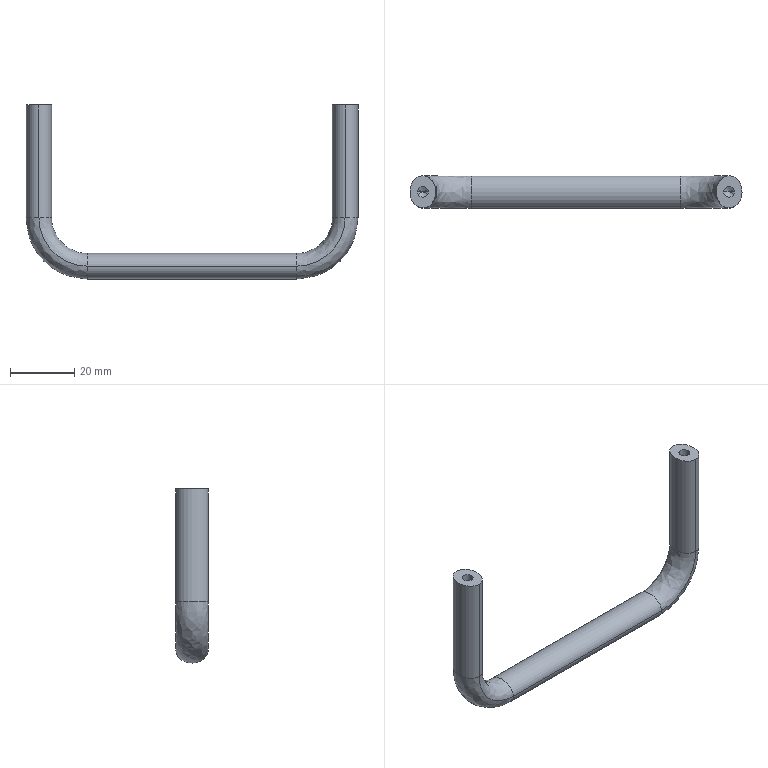Part | SolidWorks | features HoleWzd 1, Sweep 1 | 1 solid | 20 faces | box 103 x 10 x 54 mm | volume 11241 mm3 | spline 10 | cylinder 4 | cone 4 | plane 2 | commonest cylinder face diameters 3.3 x4
STEP:
#1=CARTESIAN_POINT('',(-1.65,0.,-11.5));
#2=VERTEX_POINT('',#1);
#3=CARTESIAN_POINT('',(1.65,0.,-11.5));
#4=VERTEX_POINT('',#3);
#5=CARTESIAN_POINT('',(0.,0.,-11.5));
#6=DIRECTION('',(0.,0.,1.));
#7=DIRECTION('',(1.,0.,0.));
#8=AXIS2_PLACEMENT_3D('',#5,#6,#7);
#9=CIRCLE('',#8,1.65);
#10=EDGE_CURVE('',#2,#4,#9,.T.);
#11=ORIENTED_EDGE('',*,*,#10,.F.);
#12=CARTESIAN_POINT('',(-1.65,0.,0.));
#13=VERTEX_POINT('',#12);
#14=CARTESIAN_POINT('',(-1.65,0.,0.));
#15=DIRECTION('',(0.,0.,1.));
#16=VECTOR('',#15,1000.);
#17=LINE('',#14,#16);
#18=EDGE_CURVE('',#2,#13,#17,.T.);
#19=ORIENTED_EDGE('',*,*,#18,.T.);
#20=CARTESIAN_POINT('',(1.65,0.,0.));
#21=VERTEX_POINT('',#20);
#22=CARTESIAN_POINT('',(0.,0.,0.));
#23=DIRECTION('',(0.,0.,1.));
#24=DIRECTION('',(1.,0.,0.));
#25=AXIS2_PLACEMENT_3D('',#22,#23,#24);
#26=CIRCLE('',#25,1.65);
#27=EDGE_CURVE('',#13,#21,#26,.T.);
#28=ORIENTED_EDGE('',*,*,#27,.T.);
#29=CARTESIAN_POINT('',(1.65,0.,0.));
#30=DIRECTION('',(0.,0.,1.));
#31=VECTOR('',#30,1000.);
#32=LINE('',#29,#31);
#33=EDGE_CURVE('',#4,#21,#32,.T.);
#34=ORIENTED_EDGE('',*,*,#33,.F.);
#35=EDGE_LOOP('',(#11,#19,#28,#34));
#36=FACE_OUTER_BOUND('',#35,.T.);
#37=CARTESIAN_POINT('',(0.,0.,0.));
#38=DIRECTION('',(0.,0.,1.));
#39=DIRECTION('',(1.,0.,0.));
#40=AXIS2_PLACEMENT_3D('',#37,#38,#39);
#41=CYLINDRICAL_SURFACE('',#40,1.65);
#42=ADVANCED_FACE('',(#36),#41,.F.);
#43=CARTESIAN_POINT('',(0.,0.,-12.491));
#44=VERTEX_POINT('',#43);
#45=CARTESIAN_POINT('',(1.65,0.,-11.5));
#46=DIRECTION('',(0.8572,0.,0.515));
#47=VECTOR('',#46,1000.);
#48=LINE('',#45,#47);
#49=EDGE_CURVE('',#44,#4,#48,.T.);
#50=ORIENTED_EDGE('',*,*,#49,.F.);
#51=CARTESIAN_POINT('',(-1.65,0.,-11.5));
#52=DIRECTION('',(-0.8572,0.,0.515));
#53=VECTOR('',#52,1000.);
#54=LINE('',#51,#53);
#55=EDGE_CURVE('',#44,#2,#54,.T.);
#56=ORIENTED_EDGE('',*,*,#55,.T.);
#57=ORIENTED_EDGE('',*,*,#10,.T.);
#58=EDGE_LOOP('',(#50,#56,#57));
#59=FACE_OUTER_BOUND('',#58,.T.);
#60=CARTESIAN_POINT('',(0.,0.,-11.5));
#61=DIRECTION('',(0.,0.,1.));
#62=DIRECTION('',(1.,0.,0.));
#63=AXIS2_PLACEMENT_3D('',#60,#61,#62);
#64=CONICAL_SURFACE('',#63,1.65,1.03);
#65=ADVANCED_FACE('',(#59),#64,.F.);
#66=CARTESIAN_POINT('',(93.35,0.,-11.5));
#67=VERTEX_POINT('',#66);
#68=CARTESIAN_POINT('',(96.65,0.,-11.5));
#69=VERTEX_POINT('',#68);
#70=CARTESIAN_POINT('',(95.,0.,-11.5));
#71=DIRECTION('',(0.,0.,1.));
#72=DIRECTION('',(1.,0.,0.));
#73=AXIS2_PLACEMENT_3D('',#70,#71,#72);
#74=CIRCLE('',#73,1.65);
#75=EDGE_CURVE('',#67,#69,#74,.T.);
#76=ORIENTED_EDGE('',*,*,#75,.F.);
#77=CARTESIAN_POINT('',(93.35,0.,0.));
#78=VERTEX_POINT('',#77);
#79=CARTESIAN_POINT('',(93.35,0.,0.));
#80=DIRECTION('',(0.,0.,1.));
#81=VECTOR('',#80,1000.);
#82=LINE('',#79,#81);
#83=EDGE_CURVE('',#67,#78,#82,.T.);
#84=ORIENTED_EDGE('',*,*,#83,.T.);
#85=CARTESIAN_POINT('',(96.65,0.,0.));
#86=VERTEX_POINT('',#85);
#87=CARTESIAN_POINT('',(95.,0.,0.));
#88=DIRECTION('',(0.,0.,1.));
#89=DIRECTION('',(1.,0.,0.));
#90=AXIS2_PLACEMENT_3D('',#87,#88,#89);
#91=CIRCLE('',#90,1.65);
#92=EDGE_CURVE('',#78,#86,#91,.T.);
#93=ORIENTED_EDGE('',*,*,#92,.T.);
#94=CARTESIAN_POINT('',(96.65,0.,0.));
#95=DIRECTION('',(0.,0.,1.));
#96=VECTOR('',#95,1000.);
#97=LINE('',#94,#96);
#98=EDGE_CURVE('',#69,#86,#97,.T.);
#99=ORIENTED_EDGE('',*,*,#98,.F.);
#100=EDGE_LOOP('',(#76,#84,#93,#99));
#101=FACE_OUTER_BOUND('',#100,.T.);
#102=CARTESIAN_POINT('',(95.,0.,0.));
#103=DIRECTION('',(0.,0.,1.));
#104=DIRECTION('',(1.,0.,0.));
#105=AXIS2_PLACEMENT_3D('',#102,#103,#104);
#106=CYLINDRICAL_SURFACE('',#105,1.65);
#107=ADVANCED_FACE('',(#101),#106,.F.);
#108=CARTESIAN_POINT('',(95.,0.,-12.491));
#109=VERTEX_POINT('',#108);
#110=CARTESIAN_POINT('',(96.65,0.,-11.5));
#111=DIRECTION('',(0.8572,0.,0.515));
#112=VECTOR('',#111,1000.);
#113=LINE('',#110,#112);
#114=EDGE_CURVE('',#109,#69,#113,.T.);
#115=ORIENTED_EDGE('',*,*,#114,.F.);
#116=CARTESIAN_POINT('',(93.35,0.,-11.5));
#117=DIRECTION('',(-0.8572,0.,0.515));
#118=VECTOR('',#117,1000.);
#119=LINE('',#116,#118);
#120=EDGE_CURVE('',#109,#67,#119,.T.);
#121=ORIENTED_EDGE('',*,*,#120,.T.);
#122=ORIENTED_EDGE('',*,*,#75,.T.);
#123=EDGE_LOOP('',(#115,#121,#122));
#124=FACE_OUTER_BOUND('',#123,.T.);
#125=CARTESIAN_POINT('',(95.,0.,-11.5));
#126=DIRECTION('',(0.,0.,1.));
#127=DIRECTION('',(1.,0.,0.));
#128=AXIS2_PLACEMENT_3D('',#125,#126,#127);
#129=CONICAL_SURFACE('',#128,1.65,1.03);
#130=ADVANCED_FACE('',(#124),#129,.F.);
#131=CARTESIAN_POINT('',(0.,5.,-35.));
#132=VERTEX_POINT('',#131);
#133=CARTESIAN_POINT('',(0.,-5.,-35.));
#134=VERTEX_POINT('',#133);
#135=CARTESIAN_POINT('',(0.,5.,-35.));
#136=CARTESIAN_POINT('',(-8.,5.,-35.));
#137=CARTESIAN_POINT('',(-8.,-5.,-35.));
#138=CARTESIAN_POINT('',(0.,-5.,-35.));
#139=(BOUNDED_CURVE()B_SPLINE_CURVE(3,(#135,#136,#137,#138),.UNSPECIFIED.,.F.,.F.)B_SPLINE_CURVE_WITH_KNOTS((4,4),(0.,3.142),.UNSPECIFIED.)CURVE()GEOMETRIC_REPRESENTATION_ITEM()RATIONAL_B_SPLINE_CURVE((1.,0.3333,0.3333,1.))REPRESENTATION_ITEM(''));
#140=EDGE_CURVE('',#132,#134,#139,.T.);
#141=ORIENTED_EDGE('',*,*,#140,.T.);
#142=CARTESIAN_POINT('',(0.,-5.,0.));
#143=VERTEX_POINT('',#142);
#144=CARTESIAN_POINT('',(0.,-5.,-35.));
#145=DIRECTION('',(0.,0.,1.));
#146=VECTOR('',#145,1000.);
#147=LINE('',#144,#146);
#148=EDGE_CURVE('',#134,#143,#147,.T.);
#149=ORIENTED_EDGE('',*,*,#148,.T.);
#150=CARTESIAN_POINT('',(0.,5.,0.));
#151=VERTEX_POINT('',#150);
#152=CARTESIAN_POINT('',(0.,5.,0.));
#153=CARTESIAN_POINT('',(-8.,5.,0.));
#154=CARTESIAN_POINT('',(-8.,-5.,0.));
#155=CARTESIAN_POINT('',(0.,-5.,0.));
#156=(BOUNDED_CURVE()B_SPLINE_CURVE(3,(#152,#153,#154,#155),.UNSPECIFIED.,.F.,.T.)B_SPLINE_CURVE_WITH_KNOTS((4,4),(0.,3.142),.UNSPECIFIED.)CURVE()GEOMETRIC_REPRESENTATION_ITEM()RATIONAL_B_SPLINE_CURVE((1.,0.3333,0.3333,1.))REPRESENTATION_ITEM(''));
#157=EDGE_CURVE('',#151,#143,#156,.T.);
#158=ORIENTED_EDGE('',*,*,#157,.F.);
#159=CARTESIAN_POINT('',(0.,5.,-35.));
#160=DIRECTION('',(0.,0.,1.));
#161=VECTOR('',#160,1000.);
#162=LINE('',#159,#161);
#163=EDGE_CURVE('',#132,#151,#162,.T.);
#164=ORIENTED_EDGE('',*,*,#163,.F.);
#165=EDGE_LOOP('',(#141,#149,#158,#164));
#166=FACE_OUTER_BOUND('',#165,.T.);
#167=CARTESIAN_POINT('',(0.,5.,-35.));
#168=CARTESIAN_POINT('',(0.,5.,0.));
#169=CARTESIAN_POINT('',(-8.,5.,-35.));
#170=CARTESIAN_POINT('',(-8.,5.,0.));
#171=CARTESIAN_POINT('',(-8.,-5.,-35.));
#172=CARTESIAN_POINT('',(-8.,-5.,0.));
#173=CARTESIAN_POINT('',(0.,-5.,-35.));
#174=CARTESIAN_POINT('',(0.,-5.,0.));
#175=(BOUNDED_SURFACE()B_SPLINE_SURFACE(3,1,((#167,#168),(#169,#170),(#171,#172),(#173,#174)),.UNSPECIFIED.,.F.,.F.,.T.)B_SPLINE_SURFACE_WITH_KNOTS((4,4),(2,2),(0.,1.),(0.,1.),.UNSPECIFIED.)GEOMETRIC_REPRESENTATION_ITEM()RATIONAL_B_SPLINE_SURFACE(((1.,1.),(0.3333,0.3333),(0.3333,0.3333),(1.,1.)))REPRESENTATION_ITEM('')SURFACE());
#176=ADVANCED_FACE('',(#166),#175,.T.);
#177=CARTESIAN_POINT('',(0.,-5.,-35.));
#178=CARTESIAN_POINT('',(8.,-5.,-35.));
#179=CARTESIAN_POINT('',(8.,5.,-35.));
#180=CARTESIAN_POINT('',(0.,5.,-35.));
#181=(BOUNDED_CURVE()B_SPLINE_CURVE(3,(#177,#178,#179,#180),.UNSPECIFIED.,.F.,.F.)B_SPLINE_CURVE_WITH_KNOTS((4,4),(3.142,6.283),.UNSPECIFIED.)CURVE()GEOMETRIC_REPRESENTATION_ITEM()RATIONAL_B_SPLINE_CURVE((1.,0.3333,0.3333,1.))REPRESENTATION_ITEM(''));
#182=EDGE_CURVE('',#134,#132,#181,.T.);
#183=ORIENTED_EDGE('',*,*,#182,.F.);
#184=CARTESIAN_POINT('',(15.,-5.,-50.));
#185=VERTEX_POINT('',#184);
#186=CARTESIAN_POINT('',(15.,-5.,-35.));
#187=DIRECTION('',(0.,-1.,0.));
#188=DIRECTION('',(-1.,0.,0.));
#189=AXIS2_PLACEMENT_3D('',#186,#187,#188);
#190=CIRCLE('',#189,15.);
#191=EDGE_CURVE('',#134,#185,#190,.T.);
#192=ORIENTED_EDGE('',*,*,#191,.T.);
#193=CARTESIAN_POINT('',(15.,5.,-50.));
#194=VERTEX_POINT('',#193);
#195=CARTESIAN_POINT('',(15.,-5.,-50.));
#196=CARTESIAN_POINT('',(15.,-5.,-42.));
#197=CARTESIAN_POINT('',(15.,5.,-42.));
#198=CARTESIAN_POINT('',(15.,5.,-50.));
#199=(BOUNDED_CURVE()B_SPLINE_CURVE(3,(#195,#196,#197,#198),.UNSPECIFIED.,.F.,.F.)B_SPLINE_CURVE_WITH_KNOTS((4,4),(3.142,6.283),.UNSPECIFIED.)CURVE()GEOMETRIC_REPRESENTATION_ITEM()RATIONAL_B_SPLINE_CURVE((1.,0.3333,0.3333,1.))REPRESENTATION_ITEM(''));
#200=EDGE_CURVE('',#185,#194,#199,.T.);
#201=ORIENTED_EDGE('',*,*,#200,.T.);
#202=CARTESIAN_POINT('',(15.,5.,-35.));
#203=DIRECTION('',(0.,-1.,0.));
#204=DIRECTION('',(-1.,0.,0.));
#205=AXIS2_PLACEMENT_3D('',#202,#203,#204);
#206=CIRCLE('',#205,15.);
#207=EDGE_CURVE('',#132,#194,#206,.T.);
#208=ORIENTED_EDGE('',*,*,#207,.F.);
#209=EDGE_LOOP('',(#183,#192,#201,#208));
#210=FACE_OUTER_BOUND('',#209,.T.);
#211=CARTESIAN_POINT('',(0.,-5.,-35.));
#212=CARTESIAN_POINT('',(0.,-5.,-43.787));
#213=CARTESIAN_POINT('',(6.213,-5.,-50.));
#214=CARTESIAN_POINT('',(15.,-5.,-50.));
#215=CARTESIAN_POINT('',(8.,-5.,-35.));
#216=CARTESIAN_POINT('',(8.,-5.,-39.101));
#217=CARTESIAN_POINT('',(10.899,-5.,-42.));
#218=CARTESIAN_POINT('',(15.,-5.,-42.));
#219=CARTESIAN_POINT('',(8.,5.,-35.));
#220=CARTESIAN_POINT('',(8.,5.,-39.101));
#221=CARTESIAN_POINT('',(10.899,5.,-42.));
#222=CARTESIAN_POINT('',(15.,5.,-42.));
#223=CARTESIAN_POINT('',(0.,5.,-35.));
#224=CARTESIAN_POINT('',(0.,5.,-43.787));
#225=CARTESIAN_POINT('',(6.213,5.,-50.));
#226=CARTESIAN_POINT('',(15.,5.,-50.));
#227=(BOUNDED_SURFACE()B_SPLINE_SURFACE(3,3,((#211,#212,#213,#214),(#215,#216,#217,#218),(#219,#220,#221,#222),(#223,#224,#225,#226)),.UNSPECIFIED.,.F.,.F.,.F.)B_SPLINE_SURFACE_WITH_KNOTS((4,4),(4,4),(0.,1.),(0.,1.),.UNSPECIFIED.)GEOMETRIC_REPRESENTATION_ITEM()RATIONAL_B_SPLINE_SURFACE(((1.,0.8047,0.8047,1.),(0.3333,0.2682,0.2682,0.3333),(0.3333,0.2682,0.2682,0.3333),(1.,0.8047,0.8047,1.)))REPRESENTATION_ITEM('')SURFACE());
#228=ADVANCED_FACE('',(#210),#227,.F.);
#229=ORIENTED_EDGE('',*,*,#200,.F.);
#230=CARTESIAN_POINT('',(80.,-5.,-50.));
#231=VERTEX_POINT('',#230);
#232=CARTESIAN_POINT('',(15.,-5.,-50.));
#233=DIRECTION('',(1.,0.,0.));
#234=VECTOR('',#233,1000.);
#235=LINE('',#232,#234);
#236=EDGE_CURVE('',#185,#231,#235,.T.);
#237=ORIENTED_EDGE('',*,*,#236,.T.);
#238=CARTESIAN_POINT('',(80.,5.,-50.));
#239=VERTEX_POINT('',#238);
#240=CARTESIAN_POINT('',(80.,-5.,-50.));
#241=CARTESIAN_POINT('',(80.,-5.,-42.));
#242=CARTESIAN_POINT('',(80.,5.,-42.));
#243=CARTESIAN_POINT('',(80.,5.,-50.));
#244=(BOUNDED_CURVE()B_SPLINE_CURVE(3,(#240,#241,#242,#243),.UNSPECIFIED.,.F.,.F.)B_SPLINE_CURVE_WITH_KNOTS((4,4),(3.142,6.283),.UNSPECIFIED.)CURVE()GEOMETRIC_REPRESENTATION_ITEM()RATIONAL_B_SPLINE_CURVE((1.,0.3333,0.3333,1.))REPRESENTATION_ITEM(''));
#245=EDGE_CURVE('',#231,#239,#244,.T.);
#246=ORIENTED_EDGE('',*,*,#245,.T.);
#247=CARTESIAN_POINT('',(15.,5.,-50.));
#248=DIRECTION('',(1.,0.,0.));
#249=VECTOR('',#248,1000.);
#250=LINE('',#247,#249);
#251=EDGE_CURVE('',#194,#239,#250,.T.);
#252=ORIENTED_EDGE('',*,*,#251,.F.);
#253=EDGE_LOOP('',(#229,#237,#246,#252));
#254=FACE_OUTER_BOUND('',#253,.T.);
#255=CARTESIAN_POINT('',(15.,-5.,-50.));
#256=CARTESIAN_POINT('',(80.,-5.,-50.));
#257=CARTESIAN_POINT('',(15.,-5.,-42.));
#258=CARTESIAN_POINT('',(80.,-5.,-42.));
#259=CARTESIAN_POINT('',(15.,5.,-42.));
#260=CARTESIAN_POINT('',(80.,5.,-42.));
#261=CARTESIAN_POINT('',(15.,5.,-50.));
#262=CARTESIAN_POINT('',(80.,5.,-50.));
#263=(BOUNDED_SURFACE()B_SPLINE_SURFACE(3,1,((#255,#256),(#257,#258),(#259,#260),(#261,#262)),.UNSPECIFIED.,.F.,.F.,.F.)B_SPLINE_SURFACE_WITH_KNOTS((4,4),(2,2),(0.,1.),(0.,1.),.UNSPECIFIED.)GEOMETRIC_REPRESENTATION_ITEM()RATIONAL_B_SPLINE_SURFACE(((1.,1.),(0.3333,0.3333),(0.3333,0.3333),(1.,1.)))REPRESENTATION_ITEM('')SURFACE());
#264=ADVANCED_FACE('',(#254),#263,.F.);
#265=ORIENTED_EDGE('',*,*,#245,.F.);
#266=CARTESIAN_POINT('',(95.,-5.,-35.));
#267=VERTEX_POINT('',#266);
#268=CARTESIAN_POINT('',(80.,-5.,-35.));
#269=DIRECTION('',(0.,-1.,0.));
#270=DIRECTION('',(0.,0.,-1.));
#271=AXIS2_PLACEMENT_3D('',#268,#269,#270);
#272=CIRCLE('',#271,15.);
#273=EDGE_CURVE('',#231,#267,#272,.T.);
#274=ORIENTED_EDGE('',*,*,#273,.T.);
#275=CARTESIAN_POINT('',(95.,5.,-35.));
#276=VERTEX_POINT('',#275);
#277=CARTESIAN_POINT('',(95.,-5.,-35.));
#278=CARTESIAN_POINT('',(87.,-5.,-35.));
#279=CARTESIAN_POINT('',(87.,5.,-35.));
#280=CARTESIAN_POINT('',(95.,5.,-35.));
#281=(BOUNDED_CURVE()B_SPLINE_CURVE(3,(#277,#278,#279,#280),.UNSPECIFIED.,.F.,.F.)B_SPLINE_CURVE_WITH_KNOTS((4,4),(3.142,6.283),.UNSPECIFIED.)CURVE()GEOMETRIC_REPRESENTATION_ITEM()RATIONAL_B_SPLINE_CURVE((1.,0.3333,0.3333,1.))REPRESENTATION_ITEM(''));
#282=EDGE_CURVE('',#267,#276,#281,.T.);
#283=ORIENTED_EDGE('',*,*,#282,.T.);
#284=CARTESIAN_POINT('',(80.,5.,-35.));
#285=DIRECTION('',(0.,-1.,0.));
#286=DIRECTION('',(0.,0.,-1.));
#287=AXIS2_PLACEMENT_3D('',#284,#285,#286);
#288=CIRCLE('',#287,15.);
#289=EDGE_CURVE('',#239,#276,#288,.T.);
#290=ORIENTED_EDGE('',*,*,#289,.F.);
#291=EDGE_LOOP('',(#265,#274,#283,#290));
#292=FACE_OUTER_BOUND('',#291,.T.);
#293=CARTESIAN_POINT('',(80.,-5.,-50.));
#294=CARTESIAN_POINT('',(88.787,-5.,-50.));
#295=CARTESIAN_POINT('',(95.,-5.,-43.787));
#296=CARTESIAN_POINT('',(95.,-5.,-35.));
#297=CARTESIAN_POINT('',(80.,-5.,-42.));
#298=CARTESIAN_POINT('',(84.101,-5.,-42.));
#299=CARTESIAN_POINT('',(87.,-5.,-39.101));
#300=CARTESIAN_POINT('',(87.,-5.,-35.));
#301=CARTESIAN_POINT('',(80.,5.,-42.));
#302=CARTESIAN_POINT('',(84.101,5.,-42.));
#303=CARTESIAN_POINT('',(87.,5.,-39.101));
#304=CARTESIAN_POINT('',(87.,5.,-35.));
#305=CARTESIAN_POINT('',(80.,5.,-50.));
#306=CARTESIAN_POINT('',(88.787,5.,-50.));
#307=CARTESIAN_POINT('',(95.,5.,-43.787));
#308=CARTESIAN_POINT('',(95.,5.,-35.));
#309=(BOUNDED_SURFACE()B_SPLINE_SURFACE(3,3,((#293,#294,#295,#296),(#297,#298,#299,#300),(#301,#302,#303,#304),(#305,#306,#307,#308)),.UNSPECIFIED.,.F.,.F.,.F.)B_SPLINE_SURFACE_WITH_KNOTS((4,4),(4,4),(0.,1.),(0.,1.),.UNSPECIFIED.)GEOMETRIC_REPRESENTATION_ITEM()RATIONAL_B_SPLINE_SURFACE(((1.,0.8047,0.8047,1.),(0.3333,0.2682,0.2682,0.3333),(0.3333,0.2682,0.2682,0.3333),(1.,0.8047,0.8047,1.)))REPRESENTATION_ITEM('')SURFACE());
#310=ADVANCED_FACE('',(#292),#309,.F.);
#311=ORIENTED_EDGE('',*,*,#282,.F.);
#312=CARTESIAN_POINT('',(95.,-5.,0.));
#313=VERTEX_POINT('',#312);
#314=CARTESIAN_POINT('',(95.,-5.,-35.));
#315=DIRECTION('',(0.,0.,1.));
#316=VECTOR('',#315,1000.);
#317=LINE('',#314,#316);
#318=EDGE_CURVE('',#267,#313,#317,.T.);
#319=ORIENTED_EDGE('',*,*,#318,.T.);
#320=CARTESIAN_POINT('',(95.,5.,0.));
#321=VERTEX_POINT('',#320);
#322=CARTESIAN_POINT('',(95.,-5.,0.));
#323=CARTESIAN_POINT('',(87.,-5.,0.));
#324=CARTESIAN_POINT('',(87.,5.,0.));
#325=CARTESIAN_POINT('',(95.,5.,0.));
#326=(BOUNDED_CURVE()B_SPLINE_CURVE(3,(#322,#323,#324,#325),.UNSPECIFIED.,.F.,.F.)B_SPLINE_CURVE_WITH_KNOTS((4,4),(3.142,6.283),.UNSPECIFIED.)CURVE()GEOMETRIC_REPRESENTATION_ITEM()RATIONAL_B_SPLINE_CURVE((1.,0.3333,0.3333,1.))REPRESENTATION_ITEM(''));
#327=EDGE_CURVE('',#313,#321,#326,.T.);
#328=ORIENTED_EDGE('',*,*,#327,.T.);
#329=CARTESIAN_POINT('',(95.,5.,-35.));
#330=DIRECTION('',(0.,0.,1.));
#331=VECTOR('',#330,1000.);
#332=LINE('',#329,#331);
#333=EDGE_CURVE('',#276,#321,#332,.T.);
#334=ORIENTED_EDGE('',*,*,#333,.F.);
#335=EDGE_LOOP('',(#311,#319,#328,#334));
#336=FACE_OUTER_BOUND('',#335,.T.);
#337=CARTESIAN_POINT('',(95.,-5.,-35.));
#338=CARTESIAN_POINT('',(95.,-5.,0.));
#339=CARTESIAN_POINT('',(87.,-5.,-35.));
#340=CARTESIAN_POINT('',(87.,-5.,0.));
#341=CARTESIAN_POINT('',(87.,5.,-35.));
#342=CARTESIAN_POINT('',(87.,5.,0.));
#343=CARTESIAN_POINT('',(95.,5.,-35.));
#344=CARTESIAN_POINT('',(95.,5.,0.));
#345=(BOUNDED_SURFACE()B_SPLINE_SURFACE(3,1,((#337,#338),(#339,#340),(#341,#342),(#343,#344)),.UNSPECIFIED.,.F.,.F.,.T.)B_SPLINE_SURFACE_WITH_KNOTS((4,4),(2,2),(0.,1.),(0.,1.),.UNSPECIFIED.)GEOMETRIC_REPRESENTATION_ITEM()RATIONAL_B_SPLINE_SURFACE(((1.,1.),(0.3333,0.3333),(0.3333,0.3333),(1.,1.)))REPRESENTATION_ITEM('')SURFACE());
#346=ADVANCED_FACE('',(#336),#345,.F.);
#347=CARTESIAN_POINT('',(95.,5.,0.));
#348=CARTESIAN_POINT('',(103.,5.,0.));
#349=CARTESIAN_POINT('',(103.,-5.,0.));
#350=CARTESIAN_POINT('',(95.,-5.,0.));
#351=(BOUNDED_CURVE()B_SPLINE_CURVE(3,(#347,#348,#349,#350),.UNSPECIFIED.,.F.,.F.)B_SPLINE_CURVE_WITH_KNOTS((4,4),(0.,3.142),.UNSPECIFIED.)CURVE()GEOMETRIC_REPRESENTATION_ITEM()RATIONAL_B_SPLINE_CURVE((1.,0.3333,0.3333,1.))REPRESENTATION_ITEM(''));
#352=EDGE_CURVE('',#321,#313,#351,.T.);
#353=ORIENTED_EDGE('',*,*,#352,.F.);
#354=ORIENTED_EDGE('',*,*,#327,.F.);
#355=EDGE_LOOP('',(#353,#354));
#356=FACE_OUTER_BOUND('',#355,.T.);
#357=CARTESIAN_POINT('',(95.,0.,0.));
#358=DIRECTION('',(0.,0.,1.));
#359=DIRECTION('',(1.,0.,0.));
#360=AXIS2_PLACEMENT_3D('',#357,#358,#359);
#361=CIRCLE('',#360,1.65);
#362=EDGE_CURVE('',#86,#78,#361,.T.);
#363=ORIENTED_EDGE('',*,*,#362,.F.);
#364=ORIENTED_EDGE('',*,*,#92,.F.);
#365=EDGE_LOOP('',(#363,#364));
#366=FACE_BOUND('',#365,.T.);
#367=CARTESIAN_POINT('',(95.,0.,0.));
#368=DIRECTION('',(0.,0.,-1.));
#369=DIRECTION('',(-1.,0.,0.));
#370=AXIS2_PLACEMENT_3D('',#367,#368,#369);
#371=PLANE('',#370);
#372=ADVANCED_FACE('',(#356,#366),#371,.F.);
#373=ORIENTED_EDGE('',*,*,#318,.F.);
#374=CARTESIAN_POINT('',(95.,5.,-35.));
#375=CARTESIAN_POINT('',(103.,5.,-35.));
#376=CARTESIAN_POINT('',(103.,-5.,-35.));
#377=CARTESIAN_POINT('',(95.,-5.,-35.));
#378=(BOUNDED_CURVE()B_SPLINE_CURVE(3,(#374,#375,#376,#377),.UNSPECIFIED.,.F.,.F.)B_SPLINE_CURVE_WITH_KNOTS((4,4),(0.,3.142),.UNSPECIFIED.)CURVE()GEOMETRIC_REPRESENTATION_ITEM()RATIONAL_B_SPLINE_CURVE((1.,0.3333,0.3333,1.))REPRESENTATION_ITEM(''));
#379=EDGE_CURVE('',#276,#267,#378,.T.);
#380=ORIENTED_EDGE('',*,*,#379,.F.);
#381=ORIENTED_EDGE('',*,*,#333,.T.);
#382=ORIENTED_EDGE('',*,*,#352,.T.);
#383=EDGE_LOOP('',(#373,#380,#381,#382));
#384=FACE_OUTER_BOUND('',#383,.T.);
#385=CARTESIAN_POINT('',(95.,5.,-35.));
#386=CARTESIAN_POINT('',(95.,5.,0.));
#387=CARTESIAN_POINT('',(103.,5.,-35.));
#388=CARTESIAN_POINT('',(103.,5.,0.));
#389=CARTESIAN_POINT('',(103.,-5.,-35.));
#390=CARTESIAN_POINT('',(103.,-5.,0.));
#391=CARTESIAN_POINT('',(95.,-5.,-35.));
#392=CARTESIAN_POINT('',(95.,-5.,0.));
#393=(BOUNDED_SURFACE()B_SPLINE_SURFACE(3,1,((#385,#386),(#387,#388),(#389,#390),(#391,#392)),.UNSPECIFIED.,.F.,.F.,.F.)B_SPLINE_SURFACE_WITH_KNOTS((4,4),(2,2),(0.,1.),(0.,1.),.UNSPECIFIED.)GEOMETRIC_REPRESENTATION_ITEM()RATIONAL_B_SPLINE_SURFACE(((1.,1.),(0.3333,0.3333),(0.3333,0.3333),(1.,1.)))REPRESENTATION_ITEM('')SURFACE());
#394=ADVANCED_FACE('',(#384),#393,.F.);
#395=ORIENTED_EDGE('',*,*,#273,.F.);
#396=CARTESIAN_POINT('',(80.,5.,-50.));
#397=CARTESIAN_POINT('',(80.,5.,-58.));
#398=CARTESIAN_POINT('',(80.,-5.,-58.));
#399=CARTESIAN_POINT('',(80.,-5.,-50.));
#400=(BOUNDED_CURVE()B_SPLINE_CURVE(3,(#396,#397,#398,#399),.UNSPECIFIED.,.F.,.F.)B_SPLINE_CURVE_WITH_KNOTS((4,4),(0.,3.142),.UNSPECIFIED.)CURVE()GEOMETRIC_REPRESENTATION_ITEM()RATIONAL_B_SPLINE_CURVE((1.,0.3333,0.3333,1.))REPRESENTATION_ITEM(''));
#401=EDGE_CURVE('',#239,#231,#400,.T.);
#402=ORIENTED_EDGE('',*,*,#401,.F.);
#403=ORIENTED_EDGE('',*,*,#289,.T.);
#404=ORIENTED_EDGE('',*,*,#379,.T.);
#405=EDGE_LOOP('',(#395,#402,#403,#404));
#406=FACE_OUTER_BOUND('',#405,.T.);
#407=CARTESIAN_POINT('',(80.,5.,-50.));
#408=CARTESIAN_POINT('',(88.787,5.,-50.));
#409=CARTESIAN_POINT('',(95.,5.,-43.787));
#410=CARTESIAN_POINT('',(95.,5.,-35.));
#411=CARTESIAN_POINT('',(80.,5.,-58.));
#412=CARTESIAN_POINT('',(93.473,5.,-58.));
#413=CARTESIAN_POINT('',(103.,5.,-48.473));
#414=CARTESIAN_POINT('',(103.,5.,-35.));
#415=CARTESIAN_POINT('',(80.,-5.,-58.));
#416=CARTESIAN_POINT('',(93.473,-5.,-58.));
#417=CARTESIAN_POINT('',(103.,-5.,-48.473));
#418=CARTESIAN_POINT('',(103.,-5.,-35.));
#419=CARTESIAN_POINT('',(80.,-5.,-50.));
#420=CARTESIAN_POINT('',(88.787,-5.,-50.));
#421=CARTESIAN_POINT('',(95.,-5.,-43.787));
#422=CARTESIAN_POINT('',(95.,-5.,-35.));
#423=(BOUNDED_SURFACE()B_SPLINE_SURFACE(3,3,((#407,#408,#409,#410),(#411,#412,#413,#414),(#415,#416,#417,#418),(#419,#420,#421,#422)),.UNSPECIFIED.,.F.,.F.,.F.)B_SPLINE_SURFACE_WITH_KNOTS((4,4),(4,4),(0.,1.),(0.,1.),.UNSPECIFIED.)GEOMETRIC_REPRESENTATION_ITEM()RATIONAL_B_SPLINE_SURFACE(((1.,0.8047,0.8047,1.),(0.3333,0.2682,0.2682,0.3333),(0.3333,0.2682,0.2682,0.3333),(1.,0.8047,0.8047,1.)))REPRESENTATION_ITEM('')SURFACE());
#424=ADVANCED_FACE('',(#406),#423,.F.);
#425=ORIENTED_EDGE('',*,*,#236,.F.);
#426=CARTESIAN_POINT('',(15.,5.,-50.));
#427=CARTESIAN_POINT('',(15.,5.,-58.));
#428=CARTESIAN_POINT('',(15.,-5.,-58.));
#429=CARTESIAN_POINT('',(15.,-5.,-50.));
#430=(BOUNDED_CURVE()B_SPLINE_CURVE(3,(#426,#427,#428,#429),.UNSPECIFIED.,.F.,.F.)B_SPLINE_CURVE_WITH_KNOTS((4,4),(0.,3.142),.UNSPECIFIED.)CURVE()GEOMETRIC_REPRESENTATION_ITEM()RATIONAL_B_SPLINE_CURVE((1.,0.3333,0.3333,1.))REPRESENTATION_ITEM(''));
#431=EDGE_CURVE('',#194,#185,#430,.T.);
#432=ORIENTED_EDGE('',*,*,#431,.F.);
#433=ORIENTED_EDGE('',*,*,#251,.T.);
#434=ORIENTED_EDGE('',*,*,#401,.T.);
#435=EDGE_LOOP('',(#425,#432,#433,#434));
#436=FACE_OUTER_BOUND('',#435,.T.);
#437=CARTESIAN_POINT('',(15.,5.,-50.));
#438=CARTESIAN_POINT('',(80.,5.,-50.));
#439=CARTESIAN_POINT('',(15.,5.,-58.));
#440=CARTESIAN_POINT('',(80.,5.,-58.));
#441=CARTESIAN_POINT('',(15.,-5.,-58.));
#442=CARTESIAN_POINT('',(80.,-5.,-58.));
#443=CARTESIAN_POINT('',(15.,-5.,-50.));
#444=CARTESIAN_POINT('',(80.,-5.,-50.));
#445=(BOUNDED_SURFACE()B_SPLINE_SURFACE(3,1,((#437,#438),(#439,#440),(#441,#442),(#443,#444)),.UNSPECIFIED.,.F.,.F.,.F.)B_SPLINE_SURFACE_WITH_KNOTS((4,4),(2,2),(0.,1.),(0.,1.),.UNSPECIFIED.)GEOMETRIC_REPRESENTATION_ITEM()RATIONAL_B_SPLINE_SURFACE(((1.,1.),(0.3333,0.3333),(0.3333,0.3333),(1.,1.)))REPRESENTATION_ITEM('')SURFACE());
#446=ADVANCED_FACE('',(#436),#445,.F.);
#447=ORIENTED_EDGE('',*,*,#191,.F.);
#448=ORIENTED_EDGE('',*,*,#140,.F.);
#449=ORIENTED_EDGE('',*,*,#207,.T.);
#450=ORIENTED_EDGE('',*,*,#431,.T.);
#451=EDGE_LOOP('',(#447,#448,#449,#450));
#452=FACE_OUTER_BOUND('',#451,.T.);
#453=CARTESIAN_POINT('',(0.,5.,-35.));
#454=CARTESIAN_POINT('',(0.,5.,-43.787));
#455=CARTESIAN_POINT('',(6.213,5.,-50.));
#456=CARTESIAN_POINT('',(15.,5.,-50.));
#457=CARTESIAN_POINT('',(-8.,5.,-35.));
#458=CARTESIAN_POINT('',(-8.,5.,-48.473));
#459=CARTESIAN_POINT('',(1.527,5.,-58.));
#460=CARTESIAN_POINT('',(15.,5.,-58.));
#461=CARTESIAN_POINT('',(-8.,-5.,-35.));
#462=CARTESIAN_POINT('',(-8.,-5.,-48.473));
#463=CARTESIAN_POINT('',(1.527,-5.,-58.));
#464=CARTESIAN_POINT('',(15.,-5.,-58.));
#465=CARTESIAN_POINT('',(0.,-5.,-35.));
#466=CARTESIAN_POINT('',(0.,-5.,-43.787));
#467=CARTESIAN_POINT('',(6.213,-5.,-50.));
#468=CARTESIAN_POINT('',(15.,-5.,-50.));
#469=(BOUNDED_SURFACE()B_SPLINE_SURFACE(3,3,((#453,#454,#455,#456),(#457,#458,#459,#460),(#461,#462,#463,#464),(#465,#466,#467,#468)),.UNSPECIFIED.,.F.,.F.,.T.)B_SPLINE_SURFACE_WITH_KNOTS((4,4),(4,4),(0.,1.),(0.,1.),.UNSPECIFIED.)GEOMETRIC_REPRESENTATION_ITEM()RATIONAL_B_SPLINE_SURFACE(((1.,0.8047,0.8047,1.),(0.3333,0.2682,0.2682,0.3333),(0.3333,0.2682,0.2682,0.3333),(1.,0.8047,0.8047,1.)))REPRESENTATION_ITEM('')SURFACE());
#470=ADVANCED_FACE('',(#452),#469,.F.);
#471=ORIENTED_EDGE('',*,*,#148,.F.);
#472=ORIENTED_EDGE('',*,*,#182,.T.);
#473=ORIENTED_EDGE('',*,*,#163,.T.);
#474=CARTESIAN_POINT('',(0.,-5.,0.));
#475=CARTESIAN_POINT('',(8.,-5.,0.));
#476=CARTESIAN_POINT('',(8.,5.,0.));
#477=CARTESIAN_POINT('',(0.,5.,0.));
#478=(BOUNDED_CURVE()B_SPLINE_CURVE(3,(#474,#475,#476,#477),.UNSPECIFIED.,.F.,.F.)B_SPLINE_CURVE_WITH_KNOTS((4,4),(3.142,6.283),.UNSPECIFIED.)CURVE()GEOMETRIC_REPRESENTATION_ITEM()RATIONAL_B_SPLINE_CURVE((1.,0.3333,0.3333,1.))REPRESENTATION_ITEM(''));
#479=EDGE_CURVE('',#143,#151,#478,.T.);
#480=ORIENTED_EDGE('',*,*,#479,.F.);
#481=EDGE_LOOP('',(#471,#472,#473,#480));
#482=FACE_OUTER_BOUND('',#481,.T.);
#483=CARTESIAN_POINT('',(0.,-5.,-35.));
#484=CARTESIAN_POINT('',(0.,-5.,0.));
#485=CARTESIAN_POINT('',(8.,-5.,-35.));
#486=CARTESIAN_POINT('',(8.,-5.,0.));
#487=CARTESIAN_POINT('',(8.,5.,-35.));
#488=CARTESIAN_POINT('',(8.,5.,0.));
#489=CARTESIAN_POINT('',(0.,5.,-35.));
#490=CARTESIAN_POINT('',(0.,5.,0.));
#491=(BOUNDED_SURFACE()B_SPLINE_SURFACE(3,1,((#483,#484),(#485,#486),(#487,#488),(#489,#490)),.UNSPECIFIED.,.F.,.F.,.F.)B_SPLINE_SURFACE_WITH_KNOTS((4,4),(2,2),(0.,1.),(0.,1.),.UNSPECIFIED.)GEOMETRIC_REPRESENTATION_ITEM()RATIONAL_B_SPLINE_SURFACE(((1.,1.),(0.3333,0.3333),(0.3333,0.3333),(1.,1.)))REPRESENTATION_ITEM('')SURFACE());
#492=ADVANCED_FACE('',(#482),#491,.T.);
#493=CARTESIAN_POINT('',(0.,0.,0.));
#494=DIRECTION('',(0.,0.,1.));
#495=DIRECTION('',(1.,0.,0.));
#496=AXIS2_PLACEMENT_3D('',#493,#494,#495);
#497=CIRCLE('',#496,1.65);
#498=EDGE_CURVE('',#21,#13,#497,.T.);
#499=ORIENTED_EDGE('',*,*,#498,.F.);
#500=ORIENTED_EDGE('',*,*,#27,.F.);
#501=EDGE_LOOP('',(#499,#500));
#502=FACE_BOUND('',#501,.T.);
#503=ORIENTED_EDGE('',*,*,#157,.T.);
#504=ORIENTED_EDGE('',*,*,#479,.T.);
#505=EDGE_LOOP('',(#503,#504));
#506=FACE_OUTER_BOUND('',#505,.T.);
#507=CARTESIAN_POINT('',(0.,0.,0.));
#508=DIRECTION('',(0.,0.,1.));
#509=DIRECTION('',(1.,0.,0.));
#510=AXIS2_PLACEMENT_3D('',#507,#508,#509);
#511=PLANE('',#510);
#512=ADVANCED_FACE('',(#502,#506),#511,.T.);
#513=ORIENTED_EDGE('',*,*,#120,.F.);
#514=ORIENTED_EDGE('',*,*,#114,.T.);
#515=CARTESIAN_POINT('',(95.,0.,-11.5));
#516=DIRECTION('',(0.,0.,1.));
#517=DIRECTION('',(1.,0.,0.));
#518=AXIS2_PLACEMENT_3D('',#515,#516,#517);
#519=CIRCLE('',#518,1.65);
#520=EDGE_CURVE('',#69,#67,#519,.T.);
#521=ORIENTED_EDGE('',*,*,#520,.T.);
#522=EDGE_LOOP('',(#513,#514,#521));
#523=FACE_OUTER_BOUND('',#522,.T.);
#524=CARTESIAN_POINT('',(95.,0.,-11.5));
#525=DIRECTION('',(0.,0.,1.));
#526=DIRECTION('',(1.,0.,0.));
#527=AXIS2_PLACEMENT_3D('',#524,#525,#526);
#528=CONICAL_SURFACE('',#527,1.65,1.03);
#529=ADVANCED_FACE('',(#523),#528,.F.);
#530=ORIENTED_EDGE('',*,*,#83,.F.);
#531=ORIENTED_EDGE('',*,*,#520,.F.);
#532=ORIENTED_EDGE('',*,*,#98,.T.);
#533=ORIENTED_EDGE('',*,*,#362,.T.);
#534=EDGE_LOOP('',(#530,#531,#532,#533));
#535=FACE_OUTER_BOUND('',#534,.T.);
#536=CARTESIAN_POINT('',(95.,0.,0.));
#537=DIRECTION('',(0.,0.,1.));
#538=DIRECTION('',(1.,0.,0.));
#539=AXIS2_PLACEMENT_3D('',#536,#537,#538);
#540=CYLINDRICAL_SURFACE('',#539,1.65);
#541=ADVANCED_FACE('',(#535),#540,.F.);
#542=ORIENTED_EDGE('',*,*,#55,.F.);
#543=ORIENTED_EDGE('',*,*,#49,.T.);
#544=CARTESIAN_POINT('',(0.,0.,-11.5));
#545=DIRECTION('',(0.,0.,1.));
#546=DIRECTION('',(1.,0.,0.));
#547=AXIS2_PLACEMENT_3D('',#544,#545,#546);
#548=CIRCLE('',#547,1.65);
#549=EDGE_CURVE('',#4,#2,#548,.T.);
#550=ORIENTED_EDGE('',*,*,#549,.T.);
#551=EDGE_LOOP('',(#542,#543,#550));
#552=FACE_OUTER_BOUND('',#551,.T.);
#553=CARTESIAN_POINT('',(0.,0.,-11.5));
#554=DIRECTION('',(0.,0.,1.));
#555=DIRECTION('',(1.,0.,0.));
#556=AXIS2_PLACEMENT_3D('',#553,#554,#555);
#557=CONICAL_SURFACE('',#556,1.65,1.03);
#558=ADVANCED_FACE('',(#552),#557,.F.);
#559=ORIENTED_EDGE('',*,*,#18,.F.);
#560=ORIENTED_EDGE('',*,*,#549,.F.);
#561=ORIENTED_EDGE('',*,*,#33,.T.);
#562=ORIENTED_EDGE('',*,*,#498,.T.);
#563=EDGE_LOOP('',(#559,#560,#561,#562));
#564=FACE_OUTER_BOUND('',#563,.T.);
#565=CARTESIAN_POINT('',(0.,0.,0.));
#566=DIRECTION('',(0.,0.,1.));
#567=DIRECTION('',(1.,0.,0.));
#568=AXIS2_PLACEMENT_3D('',#565,#566,#567);
#569=CYLINDRICAL_SURFACE('',#568,1.65);
#570=ADVANCED_FACE('',(#564),#569,.F.);
#571=CLOSED_SHELL('',(#42,#65,#107,#130,#176,#228,#264,#310,#346,#372,#394,#424,#446,#470,#492,#512,#529,#541,#558,#570));
#572=MANIFOLD_SOLID_BREP('',#571);
#573=CARTESIAN_POINT('',(0.,0.,0.));
#574=DIRECTION('',(0.,0.,1.));
#575=DIRECTION('',(1.,0.,0.));
#576=AXIS2_PLACEMENT_3D('',#573,#574,#575);
#577=(LENGTH_UNIT()NAMED_UNIT(*)SI_UNIT(.MILLI.,.METRE.));
#578=UNCERTAINTY_MEASURE_WITH_UNIT(LENGTH_MEASURE(0.00001),#577,'','');
#579=(NAMED_UNIT(*)PLANE_ANGLE_UNIT()SI_UNIT($,.RADIAN.));
#580=(NAMED_UNIT(*)SI_UNIT($,.STERADIAN.)SOLID_ANGLE_UNIT());
#581=(GEOMETRIC_REPRESENTATION_CONTEXT(3)GLOBAL_UNCERTAINTY_ASSIGNED_CONTEXT((#578))GLOBAL_UNIT_ASSIGNED_CONTEXT((#577,#579,#580))REPRESENTATION_CONTEXT('',''));
#582=ADVANCED_BREP_SHAPE_REPRESENTATION('',(#572,#576),#581);